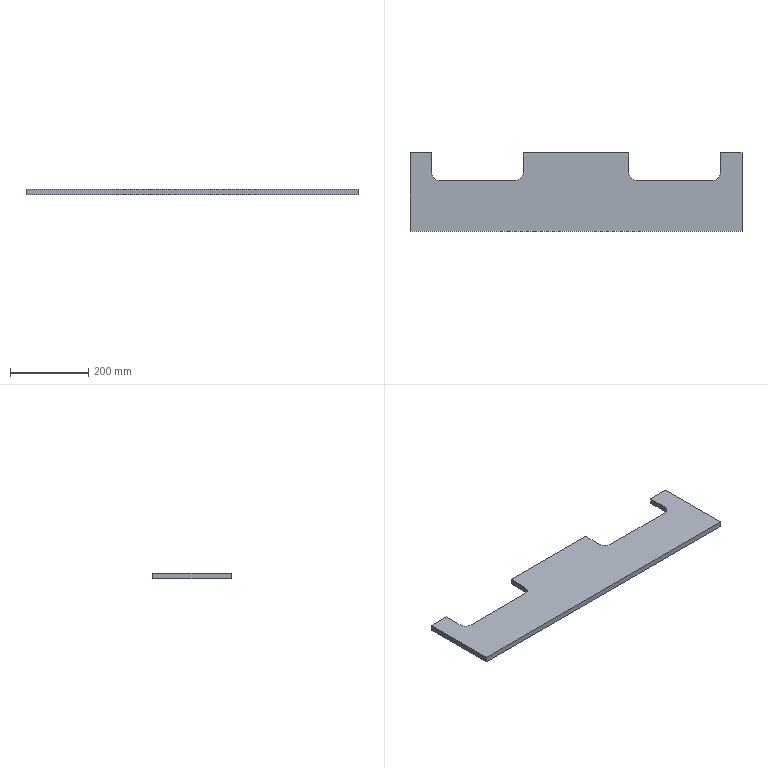Part | SolidWorks | features Cut 1, Extrusion 1, Fillet 1 | 1 solid | 18 faces | box 850 x 200 x 14 mm | volume 1924207 mm3 | plane 14 | cylinder 4 | commonest cylinder face diameters 40 x4
STEP:
#1=CARTESIAN_POINT('',(-370.,100.,14.));
#2=VERTEX_POINT('',#1);
#3=CARTESIAN_POINT('',(-425.,100.,14.));
#4=VERTEX_POINT('',#3);
#5=CARTESIAN_POINT('',(-425.,100.,14.));
#6=DIRECTION('',(-1.,0.,0.));
#7=VECTOR('',#6,1000.);
#8=LINE('',#5,#7);
#9=EDGE_CURVE('',#2,#4,#8,.T.);
#10=ORIENTED_EDGE('',*,*,#9,.F.);
#11=CARTESIAN_POINT('',(-370.,100.,0.));
#12=VERTEX_POINT('',#11);
#13=CARTESIAN_POINT('',(-370.,100.,14.001));
#14=DIRECTION('',(0.,0.,-1.));
#15=VECTOR('',#14,1000.);
#16=LINE('',#13,#15);
#17=EDGE_CURVE('',#2,#12,#16,.T.);
#18=ORIENTED_EDGE('',*,*,#17,.T.);
#19=CARTESIAN_POINT('',(-425.,100.,0.));
#20=VERTEX_POINT('',#19);
#21=CARTESIAN_POINT('',(-425.,100.,0.));
#22=DIRECTION('',(-1.,0.,0.));
#23=VECTOR('',#22,1000.);
#24=LINE('',#21,#23);
#25=EDGE_CURVE('',#12,#20,#24,.T.);
#26=ORIENTED_EDGE('',*,*,#25,.T.);
#27=CARTESIAN_POINT('',(-425.,100.,14.));
#28=DIRECTION('',(0.,0.,-1.));
#29=VECTOR('',#28,1000.);
#30=LINE('',#27,#29);
#31=EDGE_CURVE('',#4,#20,#30,.T.);
#32=ORIENTED_EDGE('',*,*,#31,.F.);
#33=EDGE_LOOP('',(#10,#18,#26,#32));
#34=FACE_OUTER_BOUND('',#33,.T.);
#35=CARTESIAN_POINT('',(-425.,100.,14.));
#36=DIRECTION('',(0.,-1.,0.));
#37=DIRECTION('',(0.,0.,-1.));
#38=AXIS2_PLACEMENT_3D('',#35,#36,#37);
#39=PLANE('',#38);
#40=ADVANCED_FACE('',(#34),#39,.F.);
#41=CARTESIAN_POINT('',(135.,100.,0.));
#42=VERTEX_POINT('',#41);
#43=CARTESIAN_POINT('',(-135.,100.,0.));
#44=VERTEX_POINT('',#43);
#45=CARTESIAN_POINT('',(-425.,100.,0.));
#46=DIRECTION('',(-1.,0.,0.));
#47=VECTOR('',#46,1000.);
#48=LINE('',#45,#47);
#49=EDGE_CURVE('',#42,#44,#48,.T.);
#50=ORIENTED_EDGE('',*,*,#49,.T.);
#51=CARTESIAN_POINT('',(-135.,100.,14.));
#52=VERTEX_POINT('',#51);
#53=CARTESIAN_POINT('',(-135.,100.,14.001));
#54=DIRECTION('',(0.,0.,-1.));
#55=VECTOR('',#54,1000.);
#56=LINE('',#53,#55);
#57=EDGE_CURVE('',#52,#44,#56,.T.);
#58=ORIENTED_EDGE('',*,*,#57,.F.);
#59=CARTESIAN_POINT('',(135.,100.,14.));
#60=VERTEX_POINT('',#59);
#61=CARTESIAN_POINT('',(-425.,100.,14.));
#62=DIRECTION('',(-1.,0.,0.));
#63=VECTOR('',#62,1000.);
#64=LINE('',#61,#63);
#65=EDGE_CURVE('',#60,#52,#64,.T.);
#66=ORIENTED_EDGE('',*,*,#65,.F.);
#67=CARTESIAN_POINT('',(135.,100.,14.001));
#68=DIRECTION('',(0.,0.,-1.));
#69=VECTOR('',#68,1000.);
#70=LINE('',#67,#69);
#71=EDGE_CURVE('',#60,#42,#70,.T.);
#72=ORIENTED_EDGE('',*,*,#71,.T.);
#73=EDGE_LOOP('',(#50,#58,#66,#72));
#74=FACE_OUTER_BOUND('',#73,.T.);
#75=CARTESIAN_POINT('',(-425.,100.,14.));
#76=DIRECTION('',(0.,-1.,0.));
#77=DIRECTION('',(0.,0.,-1.));
#78=AXIS2_PLACEMENT_3D('',#75,#76,#77);
#79=PLANE('',#78);
#80=ADVANCED_FACE('',(#74),#79,.F.);
#81=CARTESIAN_POINT('',(425.,-100.,0.));
#82=VERTEX_POINT('',#81);
#83=CARTESIAN_POINT('',(425.,100.,0.));
#84=VERTEX_POINT('',#83);
#85=CARTESIAN_POINT('',(425.,-100.,0.));
#86=DIRECTION('',(0.,1.,0.));
#87=VECTOR('',#86,1000.);
#88=LINE('',#85,#87);
#89=EDGE_CURVE('',#82,#84,#88,.T.);
#90=ORIENTED_EDGE('',*,*,#89,.T.);
#91=CARTESIAN_POINT('',(425.,100.,14.));
#92=VERTEX_POINT('',#91);
#93=CARTESIAN_POINT('',(425.,100.,14.));
#94=DIRECTION('',(0.,0.,-1.));
#95=VECTOR('',#94,1000.);
#96=LINE('',#93,#95);
#97=EDGE_CURVE('',#92,#84,#96,.T.);
#98=ORIENTED_EDGE('',*,*,#97,.F.);
#99=CARTESIAN_POINT('',(425.,-100.,14.));
#100=VERTEX_POINT('',#99);
#101=CARTESIAN_POINT('',(425.,-100.,14.));
#102=DIRECTION('',(0.,1.,0.));
#103=VECTOR('',#102,1000.);
#104=LINE('',#101,#103);
#105=EDGE_CURVE('',#100,#92,#104,.T.);
#106=ORIENTED_EDGE('',*,*,#105,.F.);
#107=CARTESIAN_POINT('',(425.,-100.,14.));
#108=DIRECTION('',(0.,0.,-1.));
#109=VECTOR('',#108,1000.);
#110=LINE('',#107,#109);
#111=EDGE_CURVE('',#100,#82,#110,.T.);
#112=ORIENTED_EDGE('',*,*,#111,.T.);
#113=EDGE_LOOP('',(#90,#98,#106,#112));
#114=FACE_OUTER_BOUND('',#113,.T.);
#115=CARTESIAN_POINT('',(425.,-100.,14.));
#116=DIRECTION('',(-1.,0.,0.));
#117=DIRECTION('',(0.,0.,1.));
#118=AXIS2_PLACEMENT_3D('',#115,#116,#117);
#119=PLANE('',#118);
#120=ADVANCED_FACE('',(#114),#119,.F.);
#121=CARTESIAN_POINT('',(370.,100.,0.));
#122=VERTEX_POINT('',#121);
#123=CARTESIAN_POINT('',(-425.,100.,0.));
#124=DIRECTION('',(-1.,0.,0.));
#125=VECTOR('',#124,1000.);
#126=LINE('',#123,#125);
#127=EDGE_CURVE('',#84,#122,#126,.T.);
#128=ORIENTED_EDGE('',*,*,#127,.T.);
#129=CARTESIAN_POINT('',(370.,100.,14.));
#130=VERTEX_POINT('',#129);
#131=CARTESIAN_POINT('',(370.,100.,14.001));
#132=DIRECTION('',(0.,0.,-1.));
#133=VECTOR('',#132,1000.);
#134=LINE('',#131,#133);
#135=EDGE_CURVE('',#130,#122,#134,.T.);
#136=ORIENTED_EDGE('',*,*,#135,.F.);
#137=CARTESIAN_POINT('',(-425.,100.,14.));
#138=DIRECTION('',(-1.,0.,0.));
#139=VECTOR('',#138,1000.);
#140=LINE('',#137,#139);
#141=EDGE_CURVE('',#92,#130,#140,.T.);
#142=ORIENTED_EDGE('',*,*,#141,.F.);
#143=ORIENTED_EDGE('',*,*,#97,.T.);
#144=EDGE_LOOP('',(#128,#136,#142,#143));
#145=FACE_OUTER_BOUND('',#144,.T.);
#146=CARTESIAN_POINT('',(-425.,100.,14.));
#147=DIRECTION('',(0.,-1.,0.));
#148=DIRECTION('',(0.,0.,-1.));
#149=AXIS2_PLACEMENT_3D('',#146,#147,#148);
#150=PLANE('',#149);
#151=ADVANCED_FACE('',(#145),#150,.F.);
#152=CARTESIAN_POINT('',(-425.,-100.,0.));
#153=VERTEX_POINT('',#152);
#154=CARTESIAN_POINT('',(-425.,-100.,0.));
#155=DIRECTION('',(0.,-1.,0.));
#156=VECTOR('',#155,1000.);
#157=LINE('',#154,#156);
#158=EDGE_CURVE('',#20,#153,#157,.T.);
#159=ORIENTED_EDGE('',*,*,#158,.T.);
#160=CARTESIAN_POINT('',(-425.,-100.,14.));
#161=VERTEX_POINT('',#160);
#162=CARTESIAN_POINT('',(-425.,-100.,14.));
#163=DIRECTION('',(0.,0.,-1.));
#164=VECTOR('',#163,1000.);
#165=LINE('',#162,#164);
#166=EDGE_CURVE('',#161,#153,#165,.T.);
#167=ORIENTED_EDGE('',*,*,#166,.F.);
#168=CARTESIAN_POINT('',(-425.,-100.,14.));
#169=DIRECTION('',(0.,-1.,0.));
#170=VECTOR('',#169,1000.);
#171=LINE('',#168,#170);
#172=EDGE_CURVE('',#4,#161,#171,.T.);
#173=ORIENTED_EDGE('',*,*,#172,.F.);
#174=ORIENTED_EDGE('',*,*,#31,.T.);
#175=EDGE_LOOP('',(#159,#167,#173,#174));
#176=FACE_OUTER_BOUND('',#175,.T.);
#177=CARTESIAN_POINT('',(-425.,-100.,14.));
#178=DIRECTION('',(1.,0.,0.));
#179=DIRECTION('',(0.,0.,-1.));
#180=AXIS2_PLACEMENT_3D('',#177,#178,#179);
#181=PLANE('',#180);
#182=ADVANCED_FACE('',(#176),#181,.F.);
#183=CARTESIAN_POINT('',(-425.,-100.,0.));
#184=DIRECTION('',(1.,0.,0.));
#185=VECTOR('',#184,1000.);
#186=LINE('',#183,#185);
#187=EDGE_CURVE('',#153,#82,#186,.T.);
#188=ORIENTED_EDGE('',*,*,#187,.T.);
#189=ORIENTED_EDGE('',*,*,#111,.F.);
#190=CARTESIAN_POINT('',(-425.,-100.,14.));
#191=DIRECTION('',(1.,0.,0.));
#192=VECTOR('',#191,1000.);
#193=LINE('',#190,#192);
#194=EDGE_CURVE('',#161,#100,#193,.T.);
#195=ORIENTED_EDGE('',*,*,#194,.F.);
#196=ORIENTED_EDGE('',*,*,#166,.T.);
#197=EDGE_LOOP('',(#188,#189,#195,#196));
#198=FACE_OUTER_BOUND('',#197,.T.);
#199=CARTESIAN_POINT('',(-425.,-100.,14.));
#200=DIRECTION('',(0.,1.,0.));
#201=DIRECTION('',(0.,0.,1.));
#202=AXIS2_PLACEMENT_3D('',#199,#200,#201);
#203=PLANE('',#202);
#204=ADVANCED_FACE('',(#198),#203,.F.);
#205=CARTESIAN_POINT('',(-350.,30.,14.));
#206=VERTEX_POINT('',#205);
#207=CARTESIAN_POINT('',(-155.,30.,14.));
#208=VERTEX_POINT('',#207);
#209=CARTESIAN_POINT('',(-370.,30.,14.));
#210=DIRECTION('',(1.,0.,0.));
#211=VECTOR('',#210,1000.);
#212=LINE('',#209,#211);
#213=EDGE_CURVE('',#206,#208,#212,.T.);
#214=ORIENTED_EDGE('',*,*,#213,.F.);
#215=CARTESIAN_POINT('',(-370.,50.,14.));
#216=VERTEX_POINT('',#215);
#217=CARTESIAN_POINT('',(-350.,50.,14.));
#218=DIRECTION('',(0.,0.,-1.));
#219=DIRECTION('',(-1.,0.,0.));
#220=AXIS2_PLACEMENT_3D('',#217,#218,#219);
#221=CIRCLE('',#220,20.);
#222=EDGE_CURVE('',#206,#216,#221,.T.);
#223=ORIENTED_EDGE('',*,*,#222,.T.);
#224=CARTESIAN_POINT('',(-370.,100.,14.));
#225=DIRECTION('',(0.,-1.,0.));
#226=VECTOR('',#225,1000.);
#227=LINE('',#224,#226);
#228=EDGE_CURVE('',#2,#216,#227,.T.);
#229=ORIENTED_EDGE('',*,*,#228,.F.);
#230=ORIENTED_EDGE('',*,*,#9,.T.);
#231=ORIENTED_EDGE('',*,*,#172,.T.);
#232=ORIENTED_EDGE('',*,*,#194,.T.);
#233=ORIENTED_EDGE('',*,*,#105,.T.);
#234=ORIENTED_EDGE('',*,*,#141,.T.);
#235=CARTESIAN_POINT('',(370.,50.,14.));
#236=VERTEX_POINT('',#235);
#237=CARTESIAN_POINT('',(370.,100.,14.));
#238=DIRECTION('',(0.,1.,0.));
#239=VECTOR('',#238,1000.);
#240=LINE('',#237,#239);
#241=EDGE_CURVE('',#236,#130,#240,.T.);
#242=ORIENTED_EDGE('',*,*,#241,.F.);
#243=CARTESIAN_POINT('',(350.,30.,14.));
#244=VERTEX_POINT('',#243);
#245=CARTESIAN_POINT('',(350.,50.,14.));
#246=DIRECTION('',(0.,0.,-1.));
#247=DIRECTION('',(-1.,0.,0.));
#248=AXIS2_PLACEMENT_3D('',#245,#246,#247);
#249=CIRCLE('',#248,20.);
#250=EDGE_CURVE('',#236,#244,#249,.T.);
#251=ORIENTED_EDGE('',*,*,#250,.T.);
#252=CARTESIAN_POINT('',(155.,30.,14.));
#253=VERTEX_POINT('',#252);
#254=CARTESIAN_POINT('',(370.,30.,14.));
#255=DIRECTION('',(1.,0.,0.));
#256=VECTOR('',#255,1000.);
#257=LINE('',#254,#256);
#258=EDGE_CURVE('',#253,#244,#257,.T.);
#259=ORIENTED_EDGE('',*,*,#258,.F.);
#260=CARTESIAN_POINT('',(135.,50.,14.));
#261=VERTEX_POINT('',#260);
#262=CARTESIAN_POINT('',(155.,50.,14.));
#263=DIRECTION('',(0.,0.,-1.));
#264=DIRECTION('',(-1.,0.,0.));
#265=AXIS2_PLACEMENT_3D('',#262,#263,#264);
#266=CIRCLE('',#265,20.);
#267=EDGE_CURVE('',#253,#261,#266,.T.);
#268=ORIENTED_EDGE('',*,*,#267,.T.);
#269=CARTESIAN_POINT('',(135.,30.,14.));
#270=DIRECTION('',(0.,-1.,0.));
#271=VECTOR('',#270,1000.);
#272=LINE('',#269,#271);
#273=EDGE_CURVE('',#60,#261,#272,.T.);
#274=ORIENTED_EDGE('',*,*,#273,.F.);
#275=ORIENTED_EDGE('',*,*,#65,.T.);
#276=CARTESIAN_POINT('',(-135.,50.,14.));
#277=VERTEX_POINT('',#276);
#278=CARTESIAN_POINT('',(-135.,30.,14.));
#279=DIRECTION('',(0.,1.,0.));
#280=VECTOR('',#279,1000.);
#281=LINE('',#278,#280);
#282=EDGE_CURVE('',#277,#52,#281,.T.);
#283=ORIENTED_EDGE('',*,*,#282,.F.);
#284=CARTESIAN_POINT('',(-155.,50.,14.));
#285=DIRECTION('',(0.,0.,-1.));
#286=DIRECTION('',(-1.,0.,0.));
#287=AXIS2_PLACEMENT_3D('',#284,#285,#286);
#288=CIRCLE('',#287,20.);
#289=EDGE_CURVE('',#277,#208,#288,.T.);
#290=ORIENTED_EDGE('',*,*,#289,.T.);
#291=EDGE_LOOP('',(#214,#223,#229,#230,#231,#232,#233,#234,#242,#251,#259,#268,#274,#275,#283,#290));
#292=FACE_OUTER_BOUND('',#291,.T.);
#293=CARTESIAN_POINT('',(0.,0.,14.));
#294=DIRECTION('',(0.,0.,-1.));
#295=DIRECTION('',(-1.,0.,0.));
#296=AXIS2_PLACEMENT_3D('',#293,#294,#295);
#297=PLANE('',#296);
#298=ADVANCED_FACE('',(#292),#297,.F.);
#299=CARTESIAN_POINT('',(-370.,50.,0.));
#300=VERTEX_POINT('',#299);
#301=CARTESIAN_POINT('',(-370.,100.,0.));
#302=DIRECTION('',(0.,1.,0.));
#303=VECTOR('',#302,1000.);
#304=LINE('',#301,#303);
#305=EDGE_CURVE('',#300,#12,#304,.T.);
#306=ORIENTED_EDGE('',*,*,#305,.F.);
#307=CARTESIAN_POINT('',(-350.,30.,0.));
#308=VERTEX_POINT('',#307);
#309=CARTESIAN_POINT('',(-350.,50.,0.));
#310=DIRECTION('',(0.,0.,1.));
#311=DIRECTION('',(-1.,0.,0.));
#312=AXIS2_PLACEMENT_3D('',#309,#310,#311);
#313=CIRCLE('',#312,20.);
#314=EDGE_CURVE('',#300,#308,#313,.T.);
#315=ORIENTED_EDGE('',*,*,#314,.T.);
#316=CARTESIAN_POINT('',(-155.,30.,0.));
#317=VERTEX_POINT('',#316);
#318=CARTESIAN_POINT('',(-370.,30.,0.));
#319=DIRECTION('',(-1.,0.,0.));
#320=VECTOR('',#319,1000.);
#321=LINE('',#318,#320);
#322=EDGE_CURVE('',#317,#308,#321,.T.);
#323=ORIENTED_EDGE('',*,*,#322,.F.);
#324=CARTESIAN_POINT('',(-135.,50.,0.));
#325=VERTEX_POINT('',#324);
#326=CARTESIAN_POINT('',(-155.,50.,0.));
#327=DIRECTION('',(0.,0.,1.));
#328=DIRECTION('',(-1.,0.,0.));
#329=AXIS2_PLACEMENT_3D('',#326,#327,#328);
#330=CIRCLE('',#329,20.);
#331=EDGE_CURVE('',#317,#325,#330,.T.);
#332=ORIENTED_EDGE('',*,*,#331,.T.);
#333=CARTESIAN_POINT('',(-135.,30.,0.));
#334=DIRECTION('',(0.,-1.,0.));
#335=VECTOR('',#334,1000.);
#336=LINE('',#333,#335);
#337=EDGE_CURVE('',#44,#325,#336,.T.);
#338=ORIENTED_EDGE('',*,*,#337,.F.);
#339=ORIENTED_EDGE('',*,*,#49,.F.);
#340=CARTESIAN_POINT('',(135.,50.,0.));
#341=VERTEX_POINT('',#340);
#342=CARTESIAN_POINT('',(135.,30.,0.));
#343=DIRECTION('',(0.,1.,0.));
#344=VECTOR('',#343,1000.);
#345=LINE('',#342,#344);
#346=EDGE_CURVE('',#341,#42,#345,.T.);
#347=ORIENTED_EDGE('',*,*,#346,.F.);
#348=CARTESIAN_POINT('',(155.,30.,0.));
#349=VERTEX_POINT('',#348);
#350=CARTESIAN_POINT('',(155.,50.,0.));
#351=DIRECTION('',(0.,0.,1.));
#352=DIRECTION('',(-1.,0.,0.));
#353=AXIS2_PLACEMENT_3D('',#350,#351,#352);
#354=CIRCLE('',#353,20.);
#355=EDGE_CURVE('',#341,#349,#354,.T.);
#356=ORIENTED_EDGE('',*,*,#355,.T.);
#357=CARTESIAN_POINT('',(350.,30.,0.));
#358=VERTEX_POINT('',#357);
#359=CARTESIAN_POINT('',(370.,30.,0.));
#360=DIRECTION('',(-1.,0.,0.));
#361=VECTOR('',#360,1000.);
#362=LINE('',#359,#361);
#363=EDGE_CURVE('',#358,#349,#362,.T.);
#364=ORIENTED_EDGE('',*,*,#363,.F.);
#365=CARTESIAN_POINT('',(370.,50.,0.));
#366=VERTEX_POINT('',#365);
#367=CARTESIAN_POINT('',(350.,50.,0.));
#368=DIRECTION('',(0.,0.,1.));
#369=DIRECTION('',(-1.,0.,0.));
#370=AXIS2_PLACEMENT_3D('',#367,#368,#369);
#371=CIRCLE('',#370,20.);
#372=EDGE_CURVE('',#358,#366,#371,.T.);
#373=ORIENTED_EDGE('',*,*,#372,.T.);
#374=CARTESIAN_POINT('',(370.,100.,0.));
#375=DIRECTION('',(0.,-1.,0.));
#376=VECTOR('',#375,1000.);
#377=LINE('',#374,#376);
#378=EDGE_CURVE('',#122,#366,#377,.T.);
#379=ORIENTED_EDGE('',*,*,#378,.F.);
#380=ORIENTED_EDGE('',*,*,#127,.F.);
#381=ORIENTED_EDGE('',*,*,#89,.F.);
#382=ORIENTED_EDGE('',*,*,#187,.F.);
#383=ORIENTED_EDGE('',*,*,#158,.F.);
#384=ORIENTED_EDGE('',*,*,#25,.F.);
#385=EDGE_LOOP('',(#306,#315,#323,#332,#338,#339,#347,#356,#364,#373,#379,#380,#381,#382,#383,#384));
#386=FACE_OUTER_BOUND('',#385,.T.);
#387=CARTESIAN_POINT('',(0.,0.,0.));
#388=DIRECTION('',(0.,0.,-1.));
#389=DIRECTION('',(-1.,0.,0.));
#390=AXIS2_PLACEMENT_3D('',#387,#388,#389);
#391=PLANE('',#390);
#392=ADVANCED_FACE('',(#386),#391,.T.);
#393=ORIENTED_EDGE('',*,*,#273,.T.);
#394=CARTESIAN_POINT('',(135.,50.,0.));
#395=DIRECTION('',(0.,0.,-1.));
#396=VECTOR('',#395,1000.);
#397=LINE('',#394,#396);
#398=EDGE_CURVE('',#261,#341,#397,.T.);
#399=ORIENTED_EDGE('',*,*,#398,.T.);
#400=ORIENTED_EDGE('',*,*,#346,.T.);
#401=ORIENTED_EDGE('',*,*,#71,.F.);
#402=EDGE_LOOP('',(#393,#399,#400,#401));
#403=FACE_OUTER_BOUND('',#402,.T.);
#404=CARTESIAN_POINT('',(135.,30.,14.001));
#405=DIRECTION('',(-1.,0.,0.));
#406=DIRECTION('',(0.,0.,1.));
#407=AXIS2_PLACEMENT_3D('',#404,#405,#406);
#408=PLANE('',#407);
#409=ADVANCED_FACE('',(#403),#408,.F.);
#410=ORIENTED_EDGE('',*,*,#258,.T.);
#411=CARTESIAN_POINT('',(350.,30.,0.));
#412=DIRECTION('',(0.,0.,-1.));
#413=VECTOR('',#412,1000.);
#414=LINE('',#411,#413);
#415=EDGE_CURVE('',#244,#358,#414,.T.);
#416=ORIENTED_EDGE('',*,*,#415,.T.);
#417=ORIENTED_EDGE('',*,*,#363,.T.);
#418=CARTESIAN_POINT('',(155.,30.,14.));
#419=DIRECTION('',(0.,0.,1.));
#420=VECTOR('',#419,1000.);
#421=LINE('',#418,#420);
#422=EDGE_CURVE('',#349,#253,#421,.T.);
#423=ORIENTED_EDGE('',*,*,#422,.T.);
#424=EDGE_LOOP('',(#410,#416,#417,#423));
#425=FACE_OUTER_BOUND('',#424,.T.);
#426=CARTESIAN_POINT('',(370.,30.,14.001));
#427=DIRECTION('',(0.,-1.,0.));
#428=DIRECTION('',(1.,0.,0.));
#429=AXIS2_PLACEMENT_3D('',#426,#427,#428);
#430=PLANE('',#429);
#431=ADVANCED_FACE('',(#425),#430,.F.);
#432=ORIENTED_EDGE('',*,*,#378,.T.);
#433=CARTESIAN_POINT('',(370.,50.,14.));
#434=DIRECTION('',(0.,0.,1.));
#435=VECTOR('',#434,1000.);
#436=LINE('',#433,#435);
#437=EDGE_CURVE('',#366,#236,#436,.T.);
#438=ORIENTED_EDGE('',*,*,#437,.T.);
#439=ORIENTED_EDGE('',*,*,#241,.T.);
#440=ORIENTED_EDGE('',*,*,#135,.T.);
#441=EDGE_LOOP('',(#432,#438,#439,#440));
#442=FACE_OUTER_BOUND('',#441,.T.);
#443=CARTESIAN_POINT('',(370.,100.,14.001));
#444=DIRECTION('',(1.,0.,0.));
#445=DIRECTION('',(0.,1.,0.));
#446=AXIS2_PLACEMENT_3D('',#443,#444,#445);
#447=PLANE('',#446);
#448=ADVANCED_FACE('',(#442),#447,.F.);
#449=ORIENTED_EDGE('',*,*,#228,.T.);
#450=CARTESIAN_POINT('',(-370.,50.,0.));
#451=DIRECTION('',(0.,0.,-1.));
#452=VECTOR('',#451,1000.);
#453=LINE('',#450,#452);
#454=EDGE_CURVE('',#216,#300,#453,.T.);
#455=ORIENTED_EDGE('',*,*,#454,.T.);
#456=ORIENTED_EDGE('',*,*,#305,.T.);
#457=ORIENTED_EDGE('',*,*,#17,.F.);
#458=EDGE_LOOP('',(#449,#455,#456,#457));
#459=FACE_OUTER_BOUND('',#458,.T.);
#460=CARTESIAN_POINT('',(-370.,100.,14.001));
#461=DIRECTION('',(-1.,0.,0.));
#462=DIRECTION('',(0.,-1.,0.));
#463=AXIS2_PLACEMENT_3D('',#460,#461,#462);
#464=PLANE('',#463);
#465=ADVANCED_FACE('',(#459),#464,.F.);
#466=ORIENTED_EDGE('',*,*,#322,.T.);
#467=CARTESIAN_POINT('',(-350.,30.,14.));
#468=DIRECTION('',(0.,0.,1.));
#469=VECTOR('',#468,1000.);
#470=LINE('',#467,#469);
#471=EDGE_CURVE('',#308,#206,#470,.T.);
#472=ORIENTED_EDGE('',*,*,#471,.T.);
#473=ORIENTED_EDGE('',*,*,#213,.T.);
#474=CARTESIAN_POINT('',(-155.,30.,0.));
#475=DIRECTION('',(0.,0.,-1.));
#476=VECTOR('',#475,1000.);
#477=LINE('',#474,#476);
#478=EDGE_CURVE('',#208,#317,#477,.T.);
#479=ORIENTED_EDGE('',*,*,#478,.T.);
#480=EDGE_LOOP('',(#466,#472,#473,#479));
#481=FACE_OUTER_BOUND('',#480,.T.);
#482=CARTESIAN_POINT('',(-370.,30.,14.001));
#483=DIRECTION('',(0.,-1.,0.));
#484=DIRECTION('',(1.,0.,0.));
#485=AXIS2_PLACEMENT_3D('',#482,#483,#484);
#486=PLANE('',#485);
#487=ADVANCED_FACE('',(#481),#486,.F.);
#488=ORIENTED_EDGE('',*,*,#337,.T.);
#489=CARTESIAN_POINT('',(-135.,50.,14.));
#490=DIRECTION('',(0.,0.,1.));
#491=VECTOR('',#490,1000.);
#492=LINE('',#489,#491);
#493=EDGE_CURVE('',#325,#277,#492,.T.);
#494=ORIENTED_EDGE('',*,*,#493,.T.);
#495=ORIENTED_EDGE('',*,*,#282,.T.);
#496=ORIENTED_EDGE('',*,*,#57,.T.);
#497=EDGE_LOOP('',(#488,#494,#495,#496));
#498=FACE_OUTER_BOUND('',#497,.T.);
#499=CARTESIAN_POINT('',(-135.,30.,14.001));
#500=DIRECTION('',(1.,0.,0.));
#501=DIRECTION('',(0.,0.,-1.));
#502=AXIS2_PLACEMENT_3D('',#499,#500,#501);
#503=PLANE('',#502);
#504=ADVANCED_FACE('',(#498),#503,.F.);
#505=ORIENTED_EDGE('',*,*,#250,.F.);
#506=ORIENTED_EDGE('',*,*,#437,.F.);
#507=ORIENTED_EDGE('',*,*,#372,.F.);
#508=ORIENTED_EDGE('',*,*,#415,.F.);
#509=EDGE_LOOP('',(#505,#506,#507,#508));
#510=FACE_OUTER_BOUND('',#509,.T.);
#511=CARTESIAN_POINT('',(350.,50.,14.001));
#512=DIRECTION('',(0.,0.,1.));
#513=DIRECTION('',(1.,0.,0.));
#514=AXIS2_PLACEMENT_3D('',#511,#512,#513);
#515=CYLINDRICAL_SURFACE('',#514,20.);
#516=ADVANCED_FACE('',(#510),#515,.F.);
#517=ORIENTED_EDGE('',*,*,#267,.F.);
#518=ORIENTED_EDGE('',*,*,#422,.F.);
#519=ORIENTED_EDGE('',*,*,#355,.F.);
#520=ORIENTED_EDGE('',*,*,#398,.F.);
#521=EDGE_LOOP('',(#517,#518,#519,#520));
#522=FACE_OUTER_BOUND('',#521,.T.);
#523=CARTESIAN_POINT('',(155.,50.,14.001));
#524=DIRECTION('',(0.,0.,1.));
#525=DIRECTION('',(1.,0.,0.));
#526=AXIS2_PLACEMENT_3D('',#523,#524,#525);
#527=CYLINDRICAL_SURFACE('',#526,20.);
#528=ADVANCED_FACE('',(#522),#527,.F.);
#529=ORIENTED_EDGE('',*,*,#222,.F.);
#530=ORIENTED_EDGE('',*,*,#471,.F.);
#531=ORIENTED_EDGE('',*,*,#314,.F.);
#532=ORIENTED_EDGE('',*,*,#454,.F.);
#533=EDGE_LOOP('',(#529,#530,#531,#532));
#534=FACE_OUTER_BOUND('',#533,.T.);
#535=CARTESIAN_POINT('',(-350.,50.,14.001));
#536=DIRECTION('',(0.,0.,1.));
#537=DIRECTION('',(1.,0.,0.));
#538=AXIS2_PLACEMENT_3D('',#535,#536,#537);
#539=CYLINDRICAL_SURFACE('',#538,20.);
#540=ADVANCED_FACE('',(#534),#539,.F.);
#541=ORIENTED_EDGE('',*,*,#289,.F.);
#542=ORIENTED_EDGE('',*,*,#493,.F.);
#543=ORIENTED_EDGE('',*,*,#331,.F.);
#544=ORIENTED_EDGE('',*,*,#478,.F.);
#545=EDGE_LOOP('',(#541,#542,#543,#544));
#546=FACE_OUTER_BOUND('',#545,.T.);
#547=CARTESIAN_POINT('',(-155.,50.,14.001));
#548=DIRECTION('',(0.,0.,1.));
#549=DIRECTION('',(1.,0.,0.));
#550=AXIS2_PLACEMENT_3D('',#547,#548,#549);
#551=CYLINDRICAL_SURFACE('',#550,20.);
#552=ADVANCED_FACE('',(#546),#551,.F.);
#553=CLOSED_SHELL('',(#40,#80,#120,#151,#182,#204,#298,#392,#409,#431,#448,#465,#487,#504,#516,#528,#540,#552));
#554=MANIFOLD_SOLID_BREP('',#553);
#555=CARTESIAN_POINT('',(0.,0.,0.));
#556=DIRECTION('',(0.,0.,1.));
#557=DIRECTION('',(1.,0.,0.));
#558=AXIS2_PLACEMENT_3D('',#555,#556,#557);
#559=(LENGTH_UNIT()NAMED_UNIT(*)SI_UNIT(.MILLI.,.METRE.));
#560=UNCERTAINTY_MEASURE_WITH_UNIT(LENGTH_MEASURE(0.00001),#559,'','');
#561=(NAMED_UNIT(*)PLANE_ANGLE_UNIT()SI_UNIT($,.RADIAN.));
#562=(NAMED_UNIT(*)SI_UNIT($,.STERADIAN.)SOLID_ANGLE_UNIT());
#563=(GEOMETRIC_REPRESENTATION_CONTEXT(3)GLOBAL_UNCERTAINTY_ASSIGNED_CONTEXT((#560))GLOBAL_UNIT_ASSIGNED_CONTEXT((#559,#561,#562))REPRESENTATION_CONTEXT('',''));
#564=ADVANCED_BREP_SHAPE_REPRESENTATION('',(#554,#558),#563);